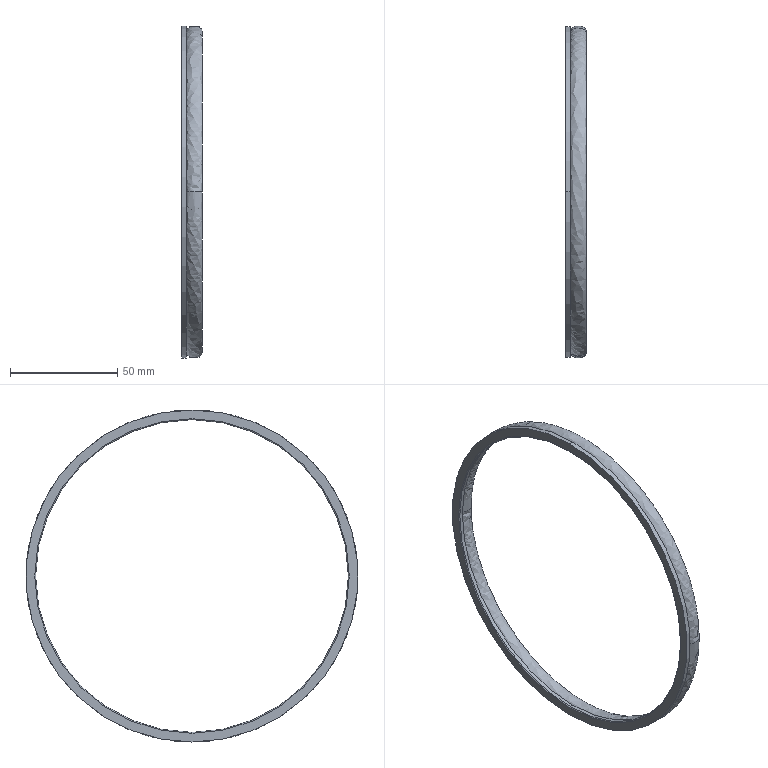Part | SolidWorks | features Revolution 3 | 2 solids | 12 faces | box 9.6 x 155 x 155 mm | volume 16985 mm3 | spline 4 | cylinder 4 | torus 2 | plane 2 | commonest cylinder face diameters 146 x2 155 x2
STEP:
#1=CARTESIAN_POINT('',(2.1,75.25,0.));
#2=VERTEX_POINT('',#1);
#3=CARTESIAN_POINT('',(2.1,-75.25,0.));
#4=VERTEX_POINT('',#3);
#5=CARTESIAN_POINT('',(2.1,0.,0.));
#6=DIRECTION('',(-1.,0.,0.));
#7=DIRECTION('',(0.,1.,0.));
#8=AXIS2_PLACEMENT_3D('',#5,#6,#7);
#9=CIRCLE('',#8,75.25);
#10=EDGE_CURVE('',#2,#4,#9,.T.);
#11=ORIENTED_EDGE('',*,*,#10,.T.);
#12=CARTESIAN_POINT('',(9.6,-75.25,0.));
#13=VERTEX_POINT('',#12);
#14=CARTESIAN_POINT('',(2.1,-75.25,0.));
#15=CARTESIAN_POINT('',(2.1,-70.75,0.));
#16=CARTESIAN_POINT('',(9.6,-70.75,0.));
#17=CARTESIAN_POINT('',(9.6,-75.25,0.));
#18=(BOUNDED_CURVE()B_SPLINE_CURVE(3,(#14,#15,#16,#17),.UNSPECIFIED.,.F.,.T.)B_SPLINE_CURVE_WITH_KNOTS((4,4),(0.,3.142),.UNSPECIFIED.)CURVE()GEOMETRIC_REPRESENTATION_ITEM()RATIONAL_B_SPLINE_CURVE((1.,0.3333,0.3333,1.))REPRESENTATION_ITEM(''));
#19=EDGE_CURVE('',#4,#13,#18,.T.);
#20=ORIENTED_EDGE('',*,*,#19,.T.);
#21=CARTESIAN_POINT('',(9.6,75.25,0.));
#22=VERTEX_POINT('',#21);
#23=CARTESIAN_POINT('',(9.6,0.,0.));
#24=DIRECTION('',(-1.,0.,0.));
#25=DIRECTION('',(0.,1.,0.));
#26=AXIS2_PLACEMENT_3D('',#23,#24,#25);
#27=CIRCLE('',#26,75.25);
#28=EDGE_CURVE('',#22,#13,#27,.T.);
#29=ORIENTED_EDGE('',*,*,#28,.F.);
#30=CARTESIAN_POINT('',(2.1,75.25,0.));
#31=CARTESIAN_POINT('',(2.1,70.75,0.));
#32=CARTESIAN_POINT('',(9.6,70.75,0.));
#33=CARTESIAN_POINT('',(9.6,75.25,0.));
#34=(BOUNDED_CURVE()B_SPLINE_CURVE(3,(#30,#31,#32,#33),.UNSPECIFIED.,.F.,.T.)B_SPLINE_CURVE_WITH_KNOTS((4,4),(0.,3.142),.UNSPECIFIED.)CURVE()GEOMETRIC_REPRESENTATION_ITEM()RATIONAL_B_SPLINE_CURVE((1.,0.3333,0.3333,1.))REPRESENTATION_ITEM(''));
#35=EDGE_CURVE('',#2,#22,#34,.T.);
#36=ORIENTED_EDGE('',*,*,#35,.F.);
#37=EDGE_LOOP('',(#11,#20,#29,#36));
#38=FACE_OUTER_BOUND('',#37,.T.);
#39=CARTESIAN_POINT('',(2.1,75.25,0.));
#40=CARTESIAN_POINT('',(2.1,75.25,-150.5));
#41=CARTESIAN_POINT('',(2.1,-75.25,-150.5));
#42=CARTESIAN_POINT('',(2.1,-75.25,0.));
#43=CARTESIAN_POINT('',(2.1,70.75,0.));
#44=CARTESIAN_POINT('',(2.1,70.75,-141.5));
#45=CARTESIAN_POINT('',(2.1,-70.75,-141.5));
#46=CARTESIAN_POINT('',(2.1,-70.75,0.));
#47=CARTESIAN_POINT('',(9.6,70.75,0.));
#48=CARTESIAN_POINT('',(9.6,70.75,-141.5));
#49=CARTESIAN_POINT('',(9.6,-70.75,-141.5));
#50=CARTESIAN_POINT('',(9.6,-70.75,0.));
#51=CARTESIAN_POINT('',(9.6,75.25,0.));
#52=CARTESIAN_POINT('',(9.6,75.25,-150.5));
#53=CARTESIAN_POINT('',(9.6,-75.25,-150.5));
#54=CARTESIAN_POINT('',(9.6,-75.25,0.));
#55=(BOUNDED_SURFACE()B_SPLINE_SURFACE(3,3,((#39,#40,#41,#42),(#43,#44,#45,#46),(#47,#48,#49,#50),(#51,#52,#53,#54)),.UNSPECIFIED.,.F.,.F.,.T.)B_SPLINE_SURFACE_WITH_KNOTS((4,4),(4,4),(0.,1.),(0.,1.),.UNSPECIFIED.)GEOMETRIC_REPRESENTATION_ITEM()RATIONAL_B_SPLINE_SURFACE(((1.,0.3333,0.3333,1.),(0.3333,0.1111,0.1111,0.3333),(0.3333,0.1111,0.1111,0.3333),(1.,0.3333,0.3333,1.)))REPRESENTATION_ITEM('')SURFACE());
#56=ADVANCED_FACE('',(#38),#55,.F.);
#57=ORIENTED_EDGE('',*,*,#28,.T.);
#58=CARTESIAN_POINT('',(9.6,-75.25,0.));
#59=CARTESIAN_POINT('',(9.6,-79.75,0.));
#60=CARTESIAN_POINT('',(2.1,-79.75,0.));
#61=CARTESIAN_POINT('',(2.1,-75.25,0.));
#62=(BOUNDED_CURVE()B_SPLINE_CURVE(3,(#58,#59,#60,#61),.UNSPECIFIED.,.F.,.T.)B_SPLINE_CURVE_WITH_KNOTS((4,4),(3.142,6.283),.UNSPECIFIED.)CURVE()GEOMETRIC_REPRESENTATION_ITEM()RATIONAL_B_SPLINE_CURVE((1.,0.3333,0.3333,1.))REPRESENTATION_ITEM(''));
#63=EDGE_CURVE('',#13,#4,#62,.T.);
#64=ORIENTED_EDGE('',*,*,#63,.T.);
#65=ORIENTED_EDGE('',*,*,#10,.F.);
#66=CARTESIAN_POINT('',(9.6,75.25,0.));
#67=CARTESIAN_POINT('',(9.6,79.75,0.));
#68=CARTESIAN_POINT('',(2.1,79.75,0.));
#69=CARTESIAN_POINT('',(2.1,75.25,0.));
#70=(BOUNDED_CURVE()B_SPLINE_CURVE(3,(#66,#67,#68,#69),.UNSPECIFIED.,.F.,.T.)B_SPLINE_CURVE_WITH_KNOTS((4,4),(3.142,6.283),.UNSPECIFIED.)CURVE()GEOMETRIC_REPRESENTATION_ITEM()RATIONAL_B_SPLINE_CURVE((1.,0.3333,0.3333,1.))REPRESENTATION_ITEM(''));
#71=EDGE_CURVE('',#22,#2,#70,.T.);
#72=ORIENTED_EDGE('',*,*,#71,.F.);
#73=EDGE_LOOP('',(#57,#64,#65,#72));
#74=FACE_OUTER_BOUND('',#73,.T.);
#75=CARTESIAN_POINT('',(9.6,75.25,0.));
#76=CARTESIAN_POINT('',(9.6,75.25,-150.5));
#77=CARTESIAN_POINT('',(9.6,-75.25,-150.5));
#78=CARTESIAN_POINT('',(9.6,-75.25,0.));
#79=CARTESIAN_POINT('',(9.6,79.75,0.));
#80=CARTESIAN_POINT('',(9.6,79.75,-159.5));
#81=CARTESIAN_POINT('',(9.6,-79.75,-159.5));
#82=CARTESIAN_POINT('',(9.6,-79.75,0.));
#83=CARTESIAN_POINT('',(2.1,79.75,0.));
#84=CARTESIAN_POINT('',(2.1,79.75,-159.5));
#85=CARTESIAN_POINT('',(2.1,-79.75,-159.5));
#86=CARTESIAN_POINT('',(2.1,-79.75,0.));
#87=CARTESIAN_POINT('',(2.1,75.25,0.));
#88=CARTESIAN_POINT('',(2.1,75.25,-150.5));
#89=CARTESIAN_POINT('',(2.1,-75.25,-150.5));
#90=CARTESIAN_POINT('',(2.1,-75.25,0.));
#91=(BOUNDED_SURFACE()B_SPLINE_SURFACE(3,3,((#75,#76,#77,#78),(#79,#80,#81,#82),(#83,#84,#85,#86),(#87,#88,#89,#90)),.UNSPECIFIED.,.F.,.F.,.T.)B_SPLINE_SURFACE_WITH_KNOTS((4,4),(4,4),(0.,1.),(0.,1.),.UNSPECIFIED.)GEOMETRIC_REPRESENTATION_ITEM()RATIONAL_B_SPLINE_SURFACE(((1.,0.3333,0.3333,1.),(0.3333,0.1111,0.1111,0.3333),(0.3333,0.1111,0.1111,0.3333),(1.,0.3333,0.3333,1.)))REPRESENTATION_ITEM('')SURFACE());
#92=ADVANCED_FACE('',(#74),#91,.F.);
#93=ORIENTED_EDGE('',*,*,#63,.F.);
#94=CARTESIAN_POINT('',(9.6,0.,0.));
#95=DIRECTION('',(-1.,0.,0.));
#96=DIRECTION('',(0.,1.,0.));
#97=AXIS2_PLACEMENT_3D('',#94,#95,#96);
#98=CIRCLE('',#97,75.25);
#99=EDGE_CURVE('',#13,#22,#98,.T.);
#100=ORIENTED_EDGE('',*,*,#99,.T.);
#101=ORIENTED_EDGE('',*,*,#71,.T.);
#102=CARTESIAN_POINT('',(2.1,0.,0.));
#103=DIRECTION('',(-1.,0.,0.));
#104=DIRECTION('',(0.,1.,0.));
#105=AXIS2_PLACEMENT_3D('',#102,#103,#104);
#106=CIRCLE('',#105,75.25);
#107=EDGE_CURVE('',#4,#2,#106,.T.);
#108=ORIENTED_EDGE('',*,*,#107,.F.);
#109=EDGE_LOOP('',(#93,#100,#101,#108));
#110=FACE_OUTER_BOUND('',#109,.T.);
#111=CARTESIAN_POINT('',(9.6,-75.25,0.));
#112=CARTESIAN_POINT('',(9.6,-75.25,150.5));
#113=CARTESIAN_POINT('',(9.6,75.25,150.5));
#114=CARTESIAN_POINT('',(9.6,75.25,0.));
#115=CARTESIAN_POINT('',(9.6,-79.75,0.));
#116=CARTESIAN_POINT('',(9.6,-79.75,159.5));
#117=CARTESIAN_POINT('',(9.6,79.75,159.5));
#118=CARTESIAN_POINT('',(9.6,79.75,0.));
#119=CARTESIAN_POINT('',(2.1,-79.75,0.));
#120=CARTESIAN_POINT('',(2.1,-79.75,159.5));
#121=CARTESIAN_POINT('',(2.1,79.75,159.5));
#122=CARTESIAN_POINT('',(2.1,79.75,0.));
#123=CARTESIAN_POINT('',(2.1,-75.25,0.));
#124=CARTESIAN_POINT('',(2.1,-75.25,150.5));
#125=CARTESIAN_POINT('',(2.1,75.25,150.5));
#126=CARTESIAN_POINT('',(2.1,75.25,0.));
#127=(BOUNDED_SURFACE()B_SPLINE_SURFACE(3,3,((#111,#112,#113,#114),(#115,#116,#117,#118),(#119,#120,#121,#122),(#123,#124,#125,#126)),.UNSPECIFIED.,.F.,.F.,.T.)B_SPLINE_SURFACE_WITH_KNOTS((4,4),(4,4),(0.,1.),(0.,1.),.UNSPECIFIED.)GEOMETRIC_REPRESENTATION_ITEM()RATIONAL_B_SPLINE_SURFACE(((1.,0.3333,0.3333,1.),(0.3333,0.1111,0.1111,0.3333),(0.3333,0.1111,0.1111,0.3333),(1.,0.3333,0.3333,1.)))REPRESENTATION_ITEM('')SURFACE());
#128=ADVANCED_FACE('',(#110),#127,.F.);
#129=ORIENTED_EDGE('',*,*,#19,.F.);
#130=ORIENTED_EDGE('',*,*,#107,.T.);
#131=ORIENTED_EDGE('',*,*,#35,.T.);
#132=ORIENTED_EDGE('',*,*,#99,.F.);
#133=EDGE_LOOP('',(#129,#130,#131,#132));
#134=FACE_OUTER_BOUND('',#133,.T.);
#135=CARTESIAN_POINT('',(2.1,-75.25,0.));
#136=CARTESIAN_POINT('',(2.1,-75.25,150.5));
#137=CARTESIAN_POINT('',(2.1,75.25,150.5));
#138=CARTESIAN_POINT('',(2.1,75.25,0.));
#139=CARTESIAN_POINT('',(2.1,-70.75,0.));
#140=CARTESIAN_POINT('',(2.1,-70.75,141.5));
#141=CARTESIAN_POINT('',(2.1,70.75,141.5));
#142=CARTESIAN_POINT('',(2.1,70.75,0.));
#143=CARTESIAN_POINT('',(9.6,-70.75,0.));
#144=CARTESIAN_POINT('',(9.6,-70.75,141.5));
#145=CARTESIAN_POINT('',(9.6,70.75,141.5));
#146=CARTESIAN_POINT('',(9.6,70.75,0.));
#147=CARTESIAN_POINT('',(9.6,-75.25,0.));
#148=CARTESIAN_POINT('',(9.6,-75.25,150.5));
#149=CARTESIAN_POINT('',(9.6,75.25,150.5));
#150=CARTESIAN_POINT('',(9.6,75.25,0.));
#151=(BOUNDED_SURFACE()B_SPLINE_SURFACE(3,3,((#135,#136,#137,#138),(#139,#140,#141,#142),(#143,#144,#145,#146),(#147,#148,#149,#150)),.UNSPECIFIED.,.F.,.F.,.T.)B_SPLINE_SURFACE_WITH_KNOTS((4,4),(4,4),(0.,1.),(0.,1.),.UNSPECIFIED.)GEOMETRIC_REPRESENTATION_ITEM()RATIONAL_B_SPLINE_SURFACE(((1.,0.3333,0.3333,1.),(0.3333,0.1111,0.1111,0.3333),(0.3333,0.1111,0.1111,0.3333),(1.,0.3333,0.3333,1.)))REPRESENTATION_ITEM('')SURFACE());
#152=ADVANCED_FACE('',(#134),#151,.F.);
#153=CLOSED_SHELL('',(#56,#92,#128,#152));
#154=MANIFOLD_SOLID_BREP('',#153);
#155=CARTESIAN_POINT('',(2.1,0.,77.5));
#156=VERTEX_POINT('',#155);
#157=CARTESIAN_POINT('',(2.1,0.,-77.5));
#158=VERTEX_POINT('',#157);
#159=CARTESIAN_POINT('',(2.1,0.,0.));
#160=DIRECTION('',(-1.,0.,0.));
#161=DIRECTION('',(0.,0.,1.));
#162=AXIS2_PLACEMENT_3D('',#159,#160,#161);
#163=CIRCLE('',#162,77.5);
#164=EDGE_CURVE('',#156,#158,#163,.T.);
#165=ORIENTED_EDGE('',*,*,#164,.T.);
#166=CARTESIAN_POINT('',(0.,0.,-77.5));
#167=VERTEX_POINT('',#166);
#168=CARTESIAN_POINT('',(-165.04,0.,-77.5));
#169=DIRECTION('',(-1.,0.,0.));
#170=VECTOR('',#169,1000.);
#171=LINE('',#168,#170);
#172=EDGE_CURVE('',#158,#167,#171,.T.);
#173=ORIENTED_EDGE('',*,*,#172,.T.);
#174=CARTESIAN_POINT('',(0.,0.,77.5));
#175=VERTEX_POINT('',#174);
#176=CARTESIAN_POINT('',(0.,0.,0.));
#177=DIRECTION('',(-1.,0.,0.));
#178=DIRECTION('',(0.,0.,1.));
#179=AXIS2_PLACEMENT_3D('',#176,#177,#178);
#180=CIRCLE('',#179,77.5);
#181=EDGE_CURVE('',#175,#167,#180,.T.);
#182=ORIENTED_EDGE('',*,*,#181,.F.);
#183=CARTESIAN_POINT('',(-165.04,0.,77.5));
#184=DIRECTION('',(-1.,0.,0.));
#185=VECTOR('',#184,1000.);
#186=LINE('',#183,#185);
#187=EDGE_CURVE('',#156,#175,#186,.T.);
#188=ORIENTED_EDGE('',*,*,#187,.F.);
#189=EDGE_LOOP('',(#165,#173,#182,#188));
#190=FACE_OUTER_BOUND('',#189,.T.);
#191=CARTESIAN_POINT('',(-165.04,0.,0.));
#192=DIRECTION('',(-1.,0.,0.));
#193=DIRECTION('',(0.,0.,1.));
#194=AXIS2_PLACEMENT_3D('',#191,#192,#193);
#195=CYLINDRICAL_SURFACE('',#194,77.5);
#196=ADVANCED_FACE('',(#190),#195,.T.);
#197=CARTESIAN_POINT('',(2.1,0.,-73.));
#198=VERTEX_POINT('',#197);
#199=CARTESIAN_POINT('',(2.1,0.,73.));
#200=VERTEX_POINT('',#199);
#201=CARTESIAN_POINT('',(2.1,0.,0.));
#202=DIRECTION('',(-1.,0.,0.));
#203=DIRECTION('',(0.,0.,1.));
#204=AXIS2_PLACEMENT_3D('',#201,#202,#203);
#205=CIRCLE('',#204,73.);
#206=EDGE_CURVE('',#198,#200,#205,.T.);
#207=ORIENTED_EDGE('',*,*,#206,.F.);
#208=CARTESIAN_POINT('',(0.4,0.,-73.));
#209=VERTEX_POINT('',#208);
#210=CARTESIAN_POINT('',(-165.04,0.,-73.));
#211=DIRECTION('',(-1.,0.,0.));
#212=VECTOR('',#211,1000.);
#213=LINE('',#210,#212);
#214=EDGE_CURVE('',#198,#209,#213,.T.);
#215=ORIENTED_EDGE('',*,*,#214,.T.);
#216=CARTESIAN_POINT('',(0.4,0.,73.));
#217=VERTEX_POINT('',#216);
#218=CARTESIAN_POINT('',(0.4,0.,0.));
#219=DIRECTION('',(-1.,0.,0.));
#220=DIRECTION('',(0.,0.,1.));
#221=AXIS2_PLACEMENT_3D('',#218,#219,#220);
#222=CIRCLE('',#221,73.);
#223=EDGE_CURVE('',#209,#217,#222,.T.);
#224=ORIENTED_EDGE('',*,*,#223,.T.);
#225=CARTESIAN_POINT('',(-165.04,0.,73.));
#226=DIRECTION('',(-1.,0.,0.));
#227=VECTOR('',#226,1000.);
#228=LINE('',#225,#227);
#229=EDGE_CURVE('',#200,#217,#228,.T.);
#230=ORIENTED_EDGE('',*,*,#229,.F.);
#231=EDGE_LOOP('',(#207,#215,#224,#230));
#232=FACE_OUTER_BOUND('',#231,.T.);
#233=CARTESIAN_POINT('',(-165.04,0.,0.));
#234=DIRECTION('',(-1.,0.,0.));
#235=DIRECTION('',(0.,0.,1.));
#236=AXIS2_PLACEMENT_3D('',#233,#234,#235);
#237=CYLINDRICAL_SURFACE('',#236,73.);
#238=ADVANCED_FACE('',(#232),#237,.F.);
#239=CARTESIAN_POINT('',(0.,0.,73.4));
#240=VERTEX_POINT('',#239);
#241=CARTESIAN_POINT('',(0.,0.,-73.4));
#242=VERTEX_POINT('',#241);
#243=CARTESIAN_POINT('',(0.,0.,0.));
#244=DIRECTION('',(-1.,0.,0.));
#245=DIRECTION('',(0.,0.,1.));
#246=AXIS2_PLACEMENT_3D('',#243,#244,#245);
#247=CIRCLE('',#246,73.4);
#248=EDGE_CURVE('',#240,#242,#247,.T.);
#249=ORIENTED_EDGE('',*,*,#248,.T.);
#250=CARTESIAN_POINT('',(0.4,0.,-73.4));
#251=DIRECTION('',(0.,1.,0.));
#252=DIRECTION('',(0.,0.,1.));
#253=AXIS2_PLACEMENT_3D('',#250,#251,#252);
#254=CIRCLE('',#253,0.4);
#255=EDGE_CURVE('',#242,#209,#254,.T.);
#256=ORIENTED_EDGE('',*,*,#255,.T.);
#257=CARTESIAN_POINT('',(0.4,0.,0.));
#258=DIRECTION('',(-1.,0.,0.));
#259=DIRECTION('',(0.,0.,1.));
#260=AXIS2_PLACEMENT_3D('',#257,#258,#259);
#261=CIRCLE('',#260,73.);
#262=EDGE_CURVE('',#217,#209,#261,.T.);
#263=ORIENTED_EDGE('',*,*,#262,.F.);
#264=CARTESIAN_POINT('',(0.4,0.,73.4));
#265=DIRECTION('',(0.,-1.,0.));
#266=DIRECTION('',(0.,0.,-1.));
#267=AXIS2_PLACEMENT_3D('',#264,#265,#266);
#268=CIRCLE('',#267,0.4);
#269=EDGE_CURVE('',#240,#217,#268,.T.);
#270=ORIENTED_EDGE('',*,*,#269,.F.);
#271=EDGE_LOOP('',(#249,#256,#263,#270));
#272=FACE_OUTER_BOUND('',#271,.T.);
#273=CARTESIAN_POINT('',(0.4,0.,0.));
#274=DIRECTION('',(-1.,0.,0.));
#275=DIRECTION('',(0.,0.,1.));
#276=AXIS2_PLACEMENT_3D('',#273,#274,#275);
#277=TOROIDAL_SURFACE('',#276,73.4,0.4);
#278=ADVANCED_FACE('',(#272),#277,.T.);
#279=ORIENTED_EDGE('',*,*,#248,.F.);
#280=CARTESIAN_POINT('',(0.,0.,0.));
#281=DIRECTION('',(-1.,0.,0.));
#282=DIRECTION('',(0.,0.,1.));
#283=AXIS2_PLACEMENT_3D('',#280,#281,#282);
#284=CIRCLE('',#283,73.4);
#285=EDGE_CURVE('',#242,#240,#284,.T.);
#286=ORIENTED_EDGE('',*,*,#285,.F.);
#287=EDGE_LOOP('',(#279,#286));
#288=FACE_BOUND('',#287,.T.);
#289=ORIENTED_EDGE('',*,*,#181,.T.);
#290=CARTESIAN_POINT('',(0.,0.,0.));
#291=DIRECTION('',(-1.,0.,0.));
#292=DIRECTION('',(0.,0.,1.));
#293=AXIS2_PLACEMENT_3D('',#290,#291,#292);
#294=CIRCLE('',#293,77.5);
#295=EDGE_CURVE('',#167,#175,#294,.T.);
#296=ORIENTED_EDGE('',*,*,#295,.T.);
#297=EDGE_LOOP('',(#289,#296));
#298=FACE_OUTER_BOUND('',#297,.T.);
#299=CARTESIAN_POINT('',(0.,0.,0.));
#300=DIRECTION('',(1.,0.,0.));
#301=DIRECTION('',(0.,0.,-1.));
#302=AXIS2_PLACEMENT_3D('',#299,#300,#301);
#303=PLANE('',#302);
#304=ADVANCED_FACE('',(#288,#298),#303,.F.);
#305=ORIENTED_EDGE('',*,*,#255,.F.);
#306=ORIENTED_EDGE('',*,*,#285,.T.);
#307=ORIENTED_EDGE('',*,*,#269,.T.);
#308=ORIENTED_EDGE('',*,*,#223,.F.);
#309=EDGE_LOOP('',(#305,#306,#307,#308));
#310=FACE_OUTER_BOUND('',#309,.T.);
#311=CARTESIAN_POINT('',(0.4,0.,0.));
#312=DIRECTION('',(-1.,0.,0.));
#313=DIRECTION('',(0.,0.,1.));
#314=AXIS2_PLACEMENT_3D('',#311,#312,#313);
#315=TOROIDAL_SURFACE('',#314,73.4,0.4);
#316=ADVANCED_FACE('',(#310),#315,.T.);
#317=ORIENTED_EDGE('',*,*,#214,.F.);
#318=CARTESIAN_POINT('',(2.1,0.,0.));
#319=DIRECTION('',(-1.,0.,0.));
#320=DIRECTION('',(0.,0.,1.));
#321=AXIS2_PLACEMENT_3D('',#318,#319,#320);
#322=CIRCLE('',#321,73.);
#323=EDGE_CURVE('',#200,#198,#322,.T.);
#324=ORIENTED_EDGE('',*,*,#323,.F.);
#325=ORIENTED_EDGE('',*,*,#229,.T.);
#326=ORIENTED_EDGE('',*,*,#262,.T.);
#327=EDGE_LOOP('',(#317,#324,#325,#326));
#328=FACE_OUTER_BOUND('',#327,.T.);
#329=CARTESIAN_POINT('',(-165.04,0.,0.));
#330=DIRECTION('',(-1.,0.,0.));
#331=DIRECTION('',(0.,0.,1.));
#332=AXIS2_PLACEMENT_3D('',#329,#330,#331);
#333=CYLINDRICAL_SURFACE('',#332,73.);
#334=ADVANCED_FACE('',(#328),#333,.F.);
#335=ORIENTED_EDGE('',*,*,#323,.T.);
#336=ORIENTED_EDGE('',*,*,#206,.T.);
#337=EDGE_LOOP('',(#335,#336));
#338=FACE_BOUND('',#337,.T.);
#339=ORIENTED_EDGE('',*,*,#164,.F.);
#340=CARTESIAN_POINT('',(2.1,0.,0.));
#341=DIRECTION('',(-1.,0.,0.));
#342=DIRECTION('',(0.,0.,1.));
#343=AXIS2_PLACEMENT_3D('',#340,#341,#342);
#344=CIRCLE('',#343,77.5);
#345=EDGE_CURVE('',#158,#156,#344,.T.);
#346=ORIENTED_EDGE('',*,*,#345,.F.);
#347=EDGE_LOOP('',(#339,#346));
#348=FACE_OUTER_BOUND('',#347,.T.);
#349=CARTESIAN_POINT('',(2.1,0.,0.));
#350=DIRECTION('',(1.,0.,0.));
#351=DIRECTION('',(0.,0.,-1.));
#352=AXIS2_PLACEMENT_3D('',#349,#350,#351);
#353=PLANE('',#352);
#354=ADVANCED_FACE('',(#338,#348),#353,.T.);
#355=ORIENTED_EDGE('',*,*,#172,.F.);
#356=ORIENTED_EDGE('',*,*,#345,.T.);
#357=ORIENTED_EDGE('',*,*,#187,.T.);
#358=ORIENTED_EDGE('',*,*,#295,.F.);
#359=EDGE_LOOP('',(#355,#356,#357,#358));
#360=FACE_OUTER_BOUND('',#359,.T.);
#361=CARTESIAN_POINT('',(-165.04,0.,0.));
#362=DIRECTION('',(-1.,0.,0.));
#363=DIRECTION('',(0.,0.,1.));
#364=AXIS2_PLACEMENT_3D('',#361,#362,#363);
#365=CYLINDRICAL_SURFACE('',#364,77.5);
#366=ADVANCED_FACE('',(#360),#365,.T.);
#367=CLOSED_SHELL('',(#196,#238,#278,#304,#316,#334,#354,#366));
#368=MANIFOLD_SOLID_BREP('',#367);
#369=CARTESIAN_POINT('',(0.,0.,0.));
#370=DIRECTION('',(0.,0.,1.));
#371=DIRECTION('',(1.,0.,0.));
#372=AXIS2_PLACEMENT_3D('',#369,#370,#371);
#373=(LENGTH_UNIT()NAMED_UNIT(*)SI_UNIT(.MILLI.,.METRE.));
#374=UNCERTAINTY_MEASURE_WITH_UNIT(LENGTH_MEASURE(0.00001),#373,'','');
#375=(NAMED_UNIT(*)PLANE_ANGLE_UNIT()SI_UNIT($,.RADIAN.));
#376=(NAMED_UNIT(*)SI_UNIT($,.STERADIAN.)SOLID_ANGLE_UNIT());
#377=(GEOMETRIC_REPRESENTATION_CONTEXT(3)GLOBAL_UNCERTAINTY_ASSIGNED_CONTEXT((#374))GLOBAL_UNIT_ASSIGNED_CONTEXT((#373,#375,#376))REPRESENTATION_CONTEXT('',''));
#378=ADVANCED_BREP_SHAPE_REPRESENTATION('',(#154,#368,#372),#377);